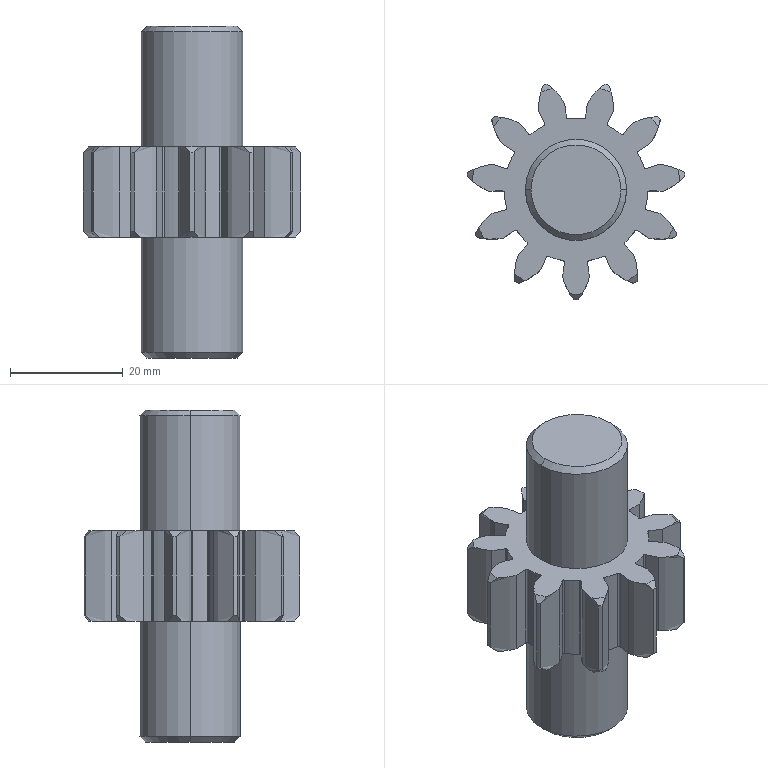Part | SolidWorks | features ICE 3, Chamfer 2, CirPattern 2, Fillet 2, Extrusion 1 | 1 solid | 127 faces | box 38.703 x 38.313 x 59 mm | volume 23395 mm3 | cylinder 53 | cone 26 | plane 26 | spline 22 | commonest cylinder face diameters 0.6 x27 25.5 x11 39 x11 18 x4